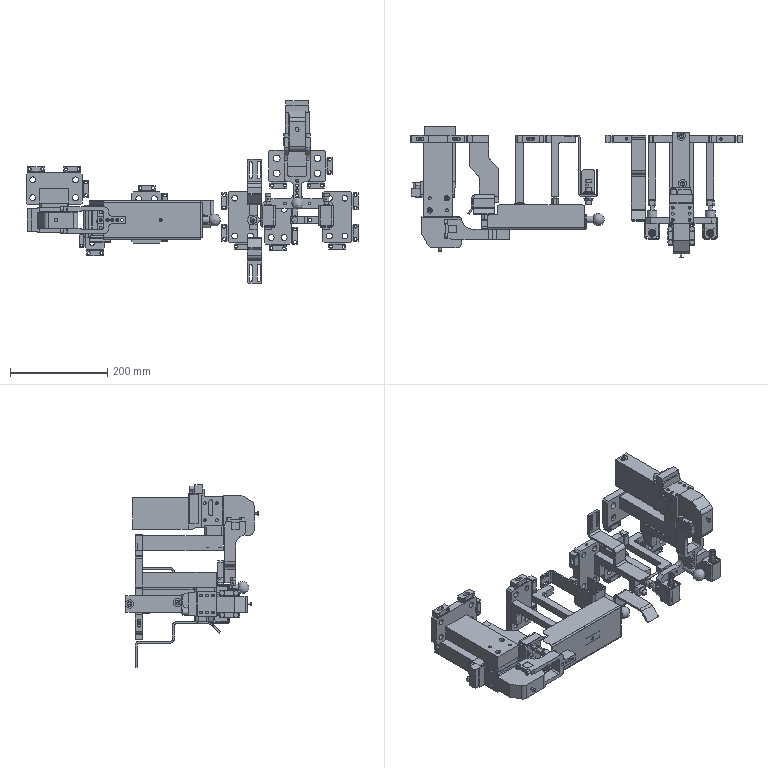Part | NX | features BREP 53 | 124 solids | 3210 faces | volume 3364887 mm3 | plane 1810 | cylinder 992 | cone 385 | sphere 9 | spline 8 | torus 6 | commonest cylinder face diameters 6 x184 6.5 x68 10 x62 7 x61 15 x58 5 x57